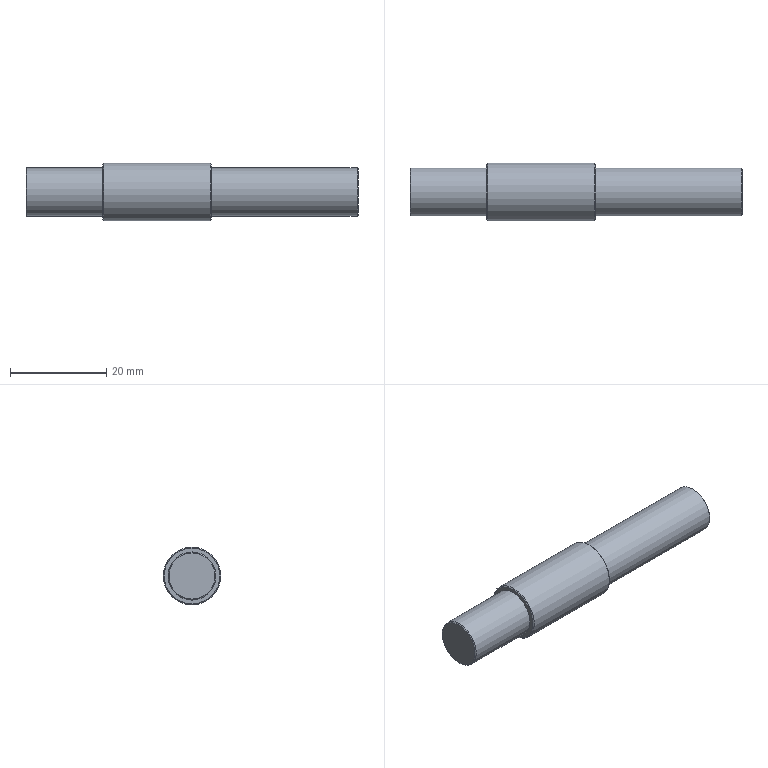Part | NX | features BREP 1 | 1 solid | 11 faces | box 69 x 12 x 12 mm | volume 6194 mm3 | cone 4 | plane 4 | cylinder 3 | commonest cylinder face diameters 10 x2 12 x1
STEP:
#1=CARTESIAN_POINT('',(38.3,0.,6.));
#2=VERTEX_POINT('',#1);
#3=CARTESIAN_POINT('',(38.3,0.,0.));
#4=DIRECTION('',(-1.,0.,0.));
#5=DIRECTION('',(0.,0.,1.));
#6=AXIS2_PLACEMENT_3D('',#3,#4,#5);
#7=CIRCLE('',#6,6.);
#8=EDGE_CURVE('',#2,#2,#7,.T.);
#9=ORIENTED_EDGE('',*,*,#8,.F.);
#10=EDGE_LOOP('',(#9));
#11=FACE_BOUND('',#10,.T.);
#12=CARTESIAN_POINT('',(38.5,0.,5.8));
#13=VERTEX_POINT('',#12);
#14=CARTESIAN_POINT('',(38.5,0.,0.));
#15=DIRECTION('',(1.,0.,0.));
#16=DIRECTION('',(0.,0.,1.));
#17=AXIS2_PLACEMENT_3D('',#14,#15,#16);
#18=CIRCLE('',#17,5.8);
#19=EDGE_CURVE('',#13,#13,#18,.T.);
#20=ORIENTED_EDGE('',*,*,#19,.F.);
#21=EDGE_LOOP('',(#20));
#22=FACE_BOUND('',#21,.T.);
#23=CARTESIAN_POINT('',(38.3,0.,0.));
#24=DIRECTION('',(-1.,0.,0.));
#25=DIRECTION('',(0.,0.,1.));
#26=AXIS2_PLACEMENT_3D('',#23,#24,#25);
#27=CONICAL_SURFACE('',#26,6.,0.7854);
#28=ADVANCED_FACE('',(#11,#22),#27,.T.);
#29=CARTESIAN_POINT('',(68.8,0.,5.));
#30=VERTEX_POINT('',#29);
#31=CARTESIAN_POINT('',(68.8,0.,0.));
#32=DIRECTION('',(-1.,0.,0.));
#33=DIRECTION('',(0.,0.,1.));
#34=AXIS2_PLACEMENT_3D('',#31,#32,#33);
#35=CIRCLE('',#34,5.);
#36=EDGE_CURVE('',#30,#30,#35,.T.);
#37=ORIENTED_EDGE('',*,*,#36,.F.);
#38=EDGE_LOOP('',(#37));
#39=FACE_BOUND('',#38,.T.);
#40=CARTESIAN_POINT('',(69.,0.,4.8));
#41=VERTEX_POINT('',#40);
#42=CARTESIAN_POINT('',(69.,0.,0.));
#43=DIRECTION('',(1.,0.,0.));
#44=DIRECTION('',(0.,0.,1.));
#45=AXIS2_PLACEMENT_3D('',#42,#43,#44);
#46=CIRCLE('',#45,4.8);
#47=EDGE_CURVE('',#41,#41,#46,.T.);
#48=ORIENTED_EDGE('',*,*,#47,.F.);
#49=EDGE_LOOP('',(#48));
#50=FACE_BOUND('',#49,.T.);
#51=CARTESIAN_POINT('',(68.8,0.,0.));
#52=DIRECTION('',(-1.,0.,0.));
#53=DIRECTION('',(0.,0.,1.));
#54=AXIS2_PLACEMENT_3D('',#51,#52,#53);
#55=CONICAL_SURFACE('',#54,5.,0.7854);
#56=ADVANCED_FACE('',(#39,#50),#55,.T.);
#57=CARTESIAN_POINT('',(0.2,0.,-5.));
#58=VERTEX_POINT('',#57);
#59=CARTESIAN_POINT('',(0.2,0.,0.));
#60=DIRECTION('',(1.,0.,0.));
#61=DIRECTION('',(0.,0.,-1.));
#62=AXIS2_PLACEMENT_3D('',#59,#60,#61);
#63=CIRCLE('',#62,5.);
#64=EDGE_CURVE('',#58,#58,#63,.T.);
#65=ORIENTED_EDGE('',*,*,#64,.F.);
#66=EDGE_LOOP('',(#65));
#67=FACE_BOUND('',#66,.T.);
#68=CARTESIAN_POINT('',(0.,0.,-4.8));
#69=VERTEX_POINT('',#68);
#70=CARTESIAN_POINT('',(0.,0.,0.));
#71=DIRECTION('',(-1.,0.,0.));
#72=DIRECTION('',(0.,0.,-1.));
#73=AXIS2_PLACEMENT_3D('',#70,#71,#72);
#74=CIRCLE('',#73,4.8);
#75=EDGE_CURVE('',#69,#69,#74,.T.);
#76=ORIENTED_EDGE('',*,*,#75,.F.);
#77=EDGE_LOOP('',(#76));
#78=FACE_BOUND('',#77,.T.);
#79=CARTESIAN_POINT('',(0.,0.,0.));
#80=DIRECTION('',(1.,0.,0.));
#81=DIRECTION('',(0.,0.,-1.));
#82=AXIS2_PLACEMENT_3D('',#79,#80,#81);
#83=CONICAL_SURFACE('',#82,4.8,0.7854);
#84=ADVANCED_FACE('',(#67,#78),#83,.T.);
#85=CARTESIAN_POINT('',(16.2,0.,6.));
#86=VERTEX_POINT('',#85);
#87=CARTESIAN_POINT('',(16.2,0.,0.));
#88=DIRECTION('',(1.,0.,0.));
#89=DIRECTION('',(0.,0.,1.));
#90=AXIS2_PLACEMENT_3D('',#87,#88,#89);
#91=CIRCLE('',#90,6.);
#92=EDGE_CURVE('',#86,#86,#91,.T.);
#93=ORIENTED_EDGE('',*,*,#92,.F.);
#94=EDGE_LOOP('',(#93));
#95=FACE_BOUND('',#94,.T.);
#96=CARTESIAN_POINT('',(16.,0.,5.8));
#97=VERTEX_POINT('',#96);
#98=CARTESIAN_POINT('',(16.,0.,0.));
#99=DIRECTION('',(-1.,0.,0.));
#100=DIRECTION('',(0.,0.,1.));
#101=AXIS2_PLACEMENT_3D('',#98,#99,#100);
#102=CIRCLE('',#101,5.8);
#103=EDGE_CURVE('',#97,#97,#102,.T.);
#104=ORIENTED_EDGE('',*,*,#103,.F.);
#105=EDGE_LOOP('',(#104));
#106=FACE_BOUND('',#105,.T.);
#107=CARTESIAN_POINT('',(16.,0.,0.));
#108=DIRECTION('',(1.,0.,0.));
#109=DIRECTION('',(0.,0.,-1.));
#110=AXIS2_PLACEMENT_3D('',#107,#108,#109);
#111=CONICAL_SURFACE('',#110,5.8,0.7854);
#112=ADVANCED_FACE('',(#95,#106),#111,.T.);
#113=ORIENTED_EDGE('',*,*,#64,.T.);
#114=EDGE_LOOP('',(#113));
#115=FACE_BOUND('',#114,.T.);
#116=CARTESIAN_POINT('',(16.,0.,5.));
#117=VERTEX_POINT('',#116);
#118=CARTESIAN_POINT('',(16.,0.,0.));
#119=DIRECTION('',(-1.,0.,0.));
#120=DIRECTION('',(0.,0.,1.));
#121=AXIS2_PLACEMENT_3D('',#118,#119,#120);
#122=CIRCLE('',#121,5.);
#123=EDGE_CURVE('',#117,#117,#122,.T.);
#124=ORIENTED_EDGE('',*,*,#123,.T.);
#125=EDGE_LOOP('',(#124));
#126=FACE_BOUND('',#125,.T.);
#127=CARTESIAN_POINT('',(16.,0.,0.));
#128=DIRECTION('',(-1.,0.,0.));
#129=DIRECTION('',(0.,0.,1.));
#130=AXIS2_PLACEMENT_3D('',#127,#128,#129);
#131=CYLINDRICAL_SURFACE('',#130,5.);
#132=ADVANCED_FACE('',(#115,#126),#131,.T.);
#133=CARTESIAN_POINT('',(38.5,0.,5.));
#134=VERTEX_POINT('',#133);
#135=CARTESIAN_POINT('',(38.5,0.,0.));
#136=DIRECTION('',(-1.,0.,0.));
#137=DIRECTION('',(0.,0.,1.));
#138=AXIS2_PLACEMENT_3D('',#135,#136,#137);
#139=CIRCLE('',#138,5.);
#140=EDGE_CURVE('',#134,#134,#139,.T.);
#141=ORIENTED_EDGE('',*,*,#140,.F.);
#142=EDGE_LOOP('',(#141));
#143=FACE_BOUND('',#142,.T.);
#144=ORIENTED_EDGE('',*,*,#36,.T.);
#145=EDGE_LOOP('',(#144));
#146=FACE_BOUND('',#145,.T.);
#147=CARTESIAN_POINT('',(0.,0.,0.));
#148=DIRECTION('',(-1.,0.,0.));
#149=DIRECTION('',(0.,0.,1.));
#150=AXIS2_PLACEMENT_3D('',#147,#148,#149);
#151=CYLINDRICAL_SURFACE('',#150,5.);
#152=ADVANCED_FACE('',(#143,#146),#151,.T.);
#153=ORIENTED_EDGE('',*,*,#92,.T.);
#154=EDGE_LOOP('',(#153));
#155=FACE_BOUND('',#154,.T.);
#156=ORIENTED_EDGE('',*,*,#8,.T.);
#157=EDGE_LOOP('',(#156));
#158=FACE_BOUND('',#157,.T.);
#159=CARTESIAN_POINT('',(0.,0.,0.));
#160=DIRECTION('',(-1.,0.,0.));
#161=DIRECTION('',(0.,0.,1.));
#162=AXIS2_PLACEMENT_3D('',#159,#160,#161);
#163=CYLINDRICAL_SURFACE('',#162,6.);
#164=ADVANCED_FACE('',(#155,#158),#163,.T.);
#165=ORIENTED_EDGE('',*,*,#19,.T.);
#166=EDGE_LOOP('',(#165));
#167=FACE_BOUND('',#166,.T.);
#168=ORIENTED_EDGE('',*,*,#140,.T.);
#169=EDGE_LOOP('',(#168));
#170=FACE_BOUND('',#169,.T.);
#171=CARTESIAN_POINT('',(38.5,6.,0.));
#172=DIRECTION('',(-1.,0.,0.));
#173=DIRECTION('',(0.,0.,1.));
#174=AXIS2_PLACEMENT_3D('',#171,#172,#173);
#175=PLANE('',#174);
#176=ADVANCED_FACE('',(#167,#170),#175,.F.);
#177=ORIENTED_EDGE('',*,*,#47,.T.);
#178=EDGE_LOOP('',(#177));
#179=FACE_BOUND('',#178,.T.);
#180=CARTESIAN_POINT('',(69.,5.,0.));
#181=DIRECTION('',(-1.,0.,0.));
#182=DIRECTION('',(0.,0.,1.));
#183=AXIS2_PLACEMENT_3D('',#180,#181,#182);
#184=PLANE('',#183);
#185=ADVANCED_FACE('',(#179),#184,.F.);
#186=ORIENTED_EDGE('',*,*,#103,.T.);
#187=EDGE_LOOP('',(#186));
#188=FACE_BOUND('',#187,.T.);
#189=ORIENTED_EDGE('',*,*,#123,.F.);
#190=EDGE_LOOP('',(#189));
#191=FACE_BOUND('',#190,.T.);
#192=CARTESIAN_POINT('',(16.,0.,0.));
#193=DIRECTION('',(-1.,0.,0.));
#194=DIRECTION('',(0.,0.,1.));
#195=AXIS2_PLACEMENT_3D('',#192,#193,#194);
#196=PLANE('',#195);
#197=ADVANCED_FACE('',(#188,#191),#196,.T.);
#198=ORIENTED_EDGE('',*,*,#75,.T.);
#199=EDGE_LOOP('',(#198));
#200=FACE_BOUND('',#199,.T.);
#201=CARTESIAN_POINT('',(0.,0.,0.));
#202=DIRECTION('',(1.,0.,0.));
#203=DIRECTION('',(0.,0.,-1.));
#204=AXIS2_PLACEMENT_3D('',#201,#202,#203);
#205=PLANE('',#204);
#206=ADVANCED_FACE('',(#200),#205,.F.);
#207=CLOSED_SHELL('',(#28,#56,#84,#112,#132,#152,#164,#176,#185,#197,#206));
#208=MANIFOLD_SOLID_BREP('',#207);
#209=(LENGTH_UNIT()NAMED_UNIT(*)SI_UNIT(.MILLI.,.METRE.));
#210=UNCERTAINTY_MEASURE_WITH_UNIT(LENGTH_MEASURE(0.00001),#209,'','');
#211=(NAMED_UNIT(*)PLANE_ANGLE_UNIT()SI_UNIT($,.RADIAN.));
#212=(NAMED_UNIT(*)SI_UNIT($,.STERADIAN.)SOLID_ANGLE_UNIT());
#213=(GEOMETRIC_REPRESENTATION_CONTEXT(3)GLOBAL_UNCERTAINTY_ASSIGNED_CONTEXT((#210))GLOBAL_UNIT_ASSIGNED_CONTEXT((#209,#211,#212))REPRESENTATION_CONTEXT('',''));
#214=ADVANCED_BREP_SHAPE_REPRESENTATION('',(#208),#213);